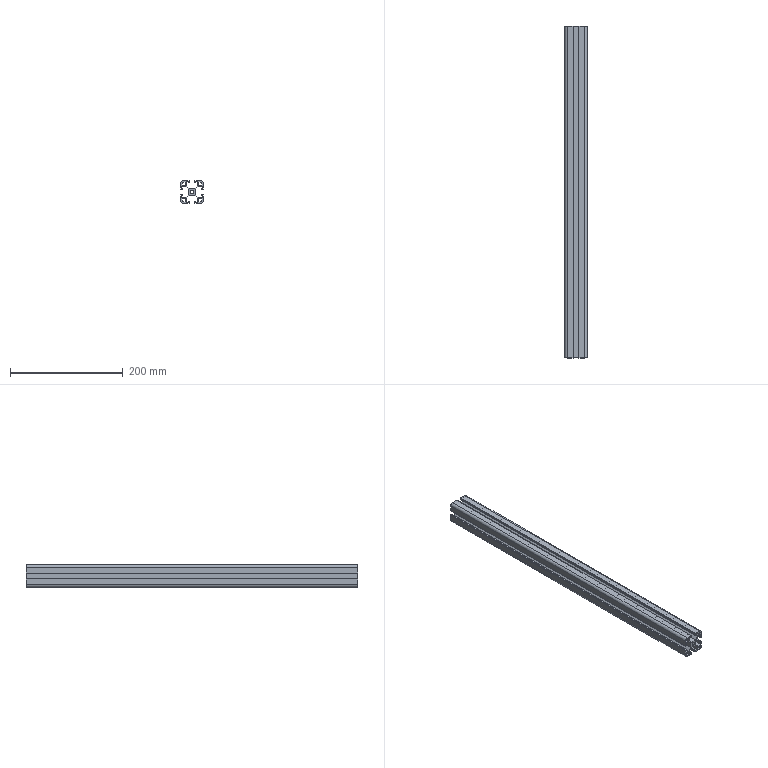Part | SolidWorks | features BaseBody 1 | 1 solid | 104 faces | box 40 x 590 x 40 mm | volume 280171 mm3 | plane 94 | cylinder 10 | commonest cylinder face diameters 5 x4 9 x4 6.8 x2